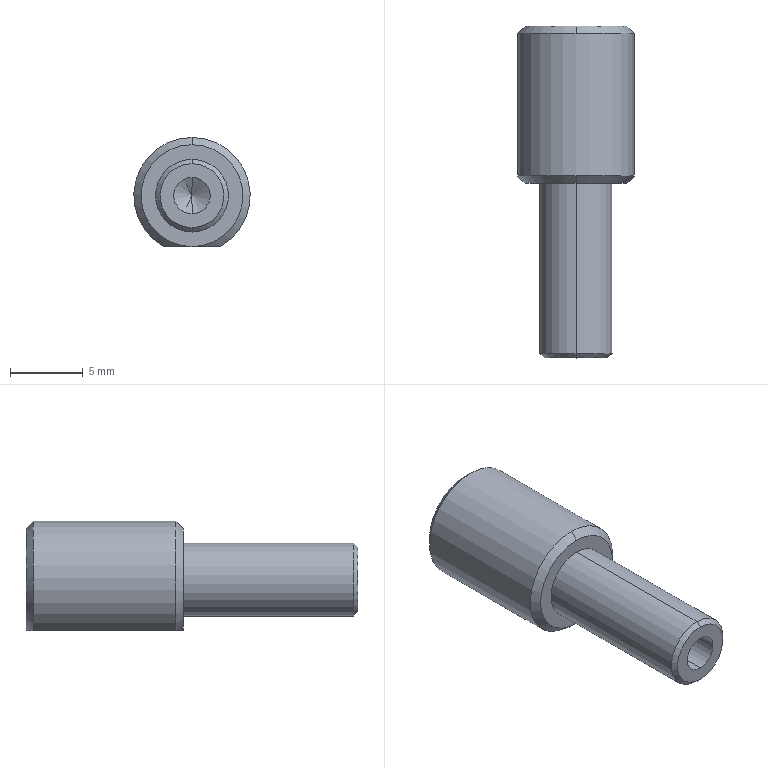Part | SolidWorks | features Chamfer 2, Cut 1, Extrusion 1, HoleWzd 1, ICE 1 | 1 solid | 17 faces | box 8 x 22.8 x 7.5 mm | volume 720.407 mm3 | cone 8 | cylinder 5 | plane 4 | commonest cylinder face diameters 2.5 x2 5 x2 8 x1
STEP:
#1=CARTESIAN_POINT('',(0.,7.5,1.25));
#2=VERTEX_POINT('',#1);
#3=CARTESIAN_POINT('',(0.,7.5,-1.25));
#4=VERTEX_POINT('',#3);
#5=CARTESIAN_POINT('',(0.,7.5,0.));
#6=DIRECTION('',(0.,-1.,0.));
#7=DIRECTION('',(0.,0.,-1.));
#8=AXIS2_PLACEMENT_3D('',#5,#6,#7);
#9=CIRCLE('',#8,1.25);
#10=EDGE_CURVE('',#2,#4,#9,.T.);
#11=ORIENTED_EDGE('',*,*,#10,.F.);
#12=CARTESIAN_POINT('',(0.,0.,1.25));
#13=VERTEX_POINT('',#12);
#14=CARTESIAN_POINT('',(0.,0.,1.25));
#15=DIRECTION('',(0.,-1.,0.));
#16=VECTOR('',#15,1000.);
#17=LINE('',#14,#16);
#18=EDGE_CURVE('',#2,#13,#17,.T.);
#19=ORIENTED_EDGE('',*,*,#18,.T.);
#20=CARTESIAN_POINT('',(0.,0.,-1.25));
#21=VERTEX_POINT('',#20);
#22=CARTESIAN_POINT('',(0.,0.,0.));
#23=DIRECTION('',(0.,-1.,0.));
#24=DIRECTION('',(0.,0.,-1.));
#25=AXIS2_PLACEMENT_3D('',#22,#23,#24);
#26=CIRCLE('',#25,1.25);
#27=EDGE_CURVE('',#13,#21,#26,.T.);
#28=ORIENTED_EDGE('',*,*,#27,.T.);
#29=CARTESIAN_POINT('',(0.,0.,-1.25));
#30=DIRECTION('',(0.,-1.,0.));
#31=VECTOR('',#30,1000.);
#32=LINE('',#29,#31);
#33=EDGE_CURVE('',#4,#21,#32,.T.);
#34=ORIENTED_EDGE('',*,*,#33,.F.);
#35=EDGE_LOOP('',(#11,#19,#28,#34));
#36=FACE_OUTER_BOUND('',#35,.T.);
#37=CARTESIAN_POINT('',(0.,0.,0.));
#38=DIRECTION('',(0.,-1.,0.));
#39=DIRECTION('',(0.,0.,-1.));
#40=AXIS2_PLACEMENT_3D('',#37,#38,#39);
#41=CYLINDRICAL_SURFACE('',#40,1.25);
#42=ADVANCED_FACE('',(#36),#41,.F.);
#43=CARTESIAN_POINT('',(0.,8.251,0.));
#44=VERTEX_POINT('',#43);
#45=CARTESIAN_POINT('',(0.,7.5,-1.25));
#46=DIRECTION('',(0.,-0.515,-0.8572));
#47=VECTOR('',#46,1000.);
#48=LINE('',#45,#47);
#49=EDGE_CURVE('',#44,#4,#48,.T.);
#50=ORIENTED_EDGE('',*,*,#49,.F.);
#51=CARTESIAN_POINT('',(0.,7.5,1.25));
#52=DIRECTION('',(0.,-0.515,0.8572));
#53=VECTOR('',#52,1000.);
#54=LINE('',#51,#53);
#55=EDGE_CURVE('',#44,#2,#54,.T.);
#56=ORIENTED_EDGE('',*,*,#55,.T.);
#57=ORIENTED_EDGE('',*,*,#10,.T.);
#58=EDGE_LOOP('',(#50,#56,#57));
#59=FACE_OUTER_BOUND('',#58,.T.);
#60=CARTESIAN_POINT('',(0.,7.5,0.));
#61=DIRECTION('',(0.,-1.,0.));
#62=DIRECTION('',(0.,0.,-1.));
#63=AXIS2_PLACEMENT_3D('',#60,#61,#62);
#64=CONICAL_SURFACE('',#63,1.25,1.03);
#65=ADVANCED_FACE('',(#59),#64,.F.);
#66=CARTESIAN_POINT('',(0.,0.,-2.2));
#67=VERTEX_POINT('',#66);
#68=CARTESIAN_POINT('',(0.,0.,2.2));
#69=VERTEX_POINT('',#68);
#70=CARTESIAN_POINT('',(0.,0.,0.));
#71=DIRECTION('',(0.,-1.,0.));
#72=DIRECTION('',(0.,0.,1.));
#73=AXIS2_PLACEMENT_3D('',#70,#71,#72);
#74=CIRCLE('',#73,2.2);
#75=EDGE_CURVE('',#67,#69,#74,.T.);
#76=ORIENTED_EDGE('',*,*,#75,.F.);
#77=CARTESIAN_POINT('',(0.,0.3,-2.5));
#78=VERTEX_POINT('',#77);
#79=CARTESIAN_POINT('',(0.,0.3,-2.5));
#80=DIRECTION('',(0.,0.7071,-0.7071));
#81=VECTOR('',#80,1000.);
#82=LINE('',#79,#81);
#83=EDGE_CURVE('',#67,#78,#82,.T.);
#84=ORIENTED_EDGE('',*,*,#83,.T.);
#85=CARTESIAN_POINT('',(0.,0.3,2.5));
#86=VERTEX_POINT('',#85);
#87=CARTESIAN_POINT('',(0.,0.3,0.));
#88=DIRECTION('',(0.,1.,0.));
#89=DIRECTION('',(0.,0.,1.));
#90=AXIS2_PLACEMENT_3D('',#87,#88,#89);
#91=CIRCLE('',#90,2.5);
#92=EDGE_CURVE('',#86,#78,#91,.T.);
#93=ORIENTED_EDGE('',*,*,#92,.F.);
#94=CARTESIAN_POINT('',(0.,0.3,2.5));
#95=DIRECTION('',(0.,0.7071,0.7071));
#96=VECTOR('',#95,1000.);
#97=LINE('',#94,#96);
#98=EDGE_CURVE('',#69,#86,#97,.T.);
#99=ORIENTED_EDGE('',*,*,#98,.F.);
#100=EDGE_LOOP('',(#76,#84,#93,#99));
#101=FACE_OUTER_BOUND('',#100,.T.);
#102=CARTESIAN_POINT('',(0.,0.3,0.));
#103=DIRECTION('',(0.,1.,0.));
#104=DIRECTION('',(0.,0.,1.));
#105=AXIS2_PLACEMENT_3D('',#102,#103,#104);
#106=CONICAL_SURFACE('',#105,2.5,0.7854);
#107=ADVANCED_FACE('',(#101),#106,.T.);
#108=CARTESIAN_POINT('',(0.,12.,3.5));
#109=VERTEX_POINT('',#108);
#110=CARTESIAN_POINT('',(0.,12.,-3.5));
#111=VERTEX_POINT('',#110);
#112=CARTESIAN_POINT('',(0.,12.,0.));
#113=DIRECTION('',(0.,-1.,0.));
#114=DIRECTION('',(0.,0.,1.));
#115=AXIS2_PLACEMENT_3D('',#112,#113,#114);
#116=CIRCLE('',#115,3.5);
#117=EDGE_CURVE('',#109,#111,#116,.T.);
#118=ORIENTED_EDGE('',*,*,#117,.F.);
#119=CARTESIAN_POINT('',(0.,12.5,4.));
#120=VERTEX_POINT('',#119);
#121=CARTESIAN_POINT('',(0.,12.5,4.));
#122=DIRECTION('',(0.,0.7071,0.7071));
#123=VECTOR('',#122,1000.);
#124=LINE('',#121,#123);
#125=EDGE_CURVE('',#109,#120,#124,.T.);
#126=ORIENTED_EDGE('',*,*,#125,.T.);
#127=CARTESIAN_POINT('',(-1.936,12.5,-3.5));
#128=VERTEX_POINT('',#127);
#129=CARTESIAN_POINT('',(0.,12.5,0.));
#130=DIRECTION('',(0.,1.,0.));
#131=DIRECTION('',(0.,0.,1.));
#132=AXIS2_PLACEMENT_3D('',#129,#130,#131);
#133=CIRCLE('',#132,4.);
#134=EDGE_CURVE('',#128,#120,#133,.T.);
#135=ORIENTED_EDGE('',*,*,#134,.F.);
#136=CARTESIAN_POINT('',(0.,12.,-3.5));
#137=CARTESIAN_POINT('',(-0.34,12.,-3.5));
#138=CARTESIAN_POINT('',(-0.673,12.05,-3.5));
#139=CARTESIAN_POINT('',(-1.328,12.23,-3.5));
#140=CARTESIAN_POINT('',(-1.638,12.355,-3.5));
#141=CARTESIAN_POINT('',(-1.936,12.5,-3.5));
#142=B_SPLINE_CURVE_WITH_KNOTS('',3,(#136,#137,#138,#139,#140,#141),.UNSPECIFIED.,.F.,.F.,(4,2,4),(0.004182,0.005183,0.006184),.UNSPECIFIED.);
#143=EDGE_CURVE('',#111,#128,#142,.T.);
#144=ORIENTED_EDGE('',*,*,#143,.F.);
#145=EDGE_LOOP('',(#118,#126,#135,#144));
#146=FACE_OUTER_BOUND('',#145,.T.);
#147=CARTESIAN_POINT('',(0.,12.5,0.));
#148=DIRECTION('',(0.,1.,0.));
#149=DIRECTION('',(0.,0.,1.));
#150=AXIS2_PLACEMENT_3D('',#147,#148,#149);
#151=CONICAL_SURFACE('',#150,4.,0.7854);
#152=ADVANCED_FACE('',(#146),#151,.T.);
#153=CARTESIAN_POINT('',(0.,22.8,3.5));
#154=VERTEX_POINT('',#153);
#155=CARTESIAN_POINT('',(0.,22.8,-3.5));
#156=VERTEX_POINT('',#155);
#157=CARTESIAN_POINT('',(0.,22.8,0.));
#158=DIRECTION('',(0.,1.,0.));
#159=DIRECTION('',(0.,0.,1.));
#160=AXIS2_PLACEMENT_3D('',#157,#158,#159);
#161=CIRCLE('',#160,3.5);
#162=EDGE_CURVE('',#154,#156,#161,.T.);
#163=ORIENTED_EDGE('',*,*,#162,.F.);
#164=CARTESIAN_POINT('',(0.,22.3,4.));
#165=VERTEX_POINT('',#164);
#166=CARTESIAN_POINT('',(0.,22.8,3.5));
#167=DIRECTION('',(0.,-0.7071,0.7071));
#168=VECTOR('',#167,1000.);
#169=LINE('',#166,#168);
#170=EDGE_CURVE('',#154,#165,#169,.T.);
#171=ORIENTED_EDGE('',*,*,#170,.T.);
#172=CARTESIAN_POINT('',(1.936,22.3,-3.5));
#173=VERTEX_POINT('',#172);
#174=CARTESIAN_POINT('',(0.,22.3,0.));
#175=DIRECTION('',(0.,-1.,0.));
#176=DIRECTION('',(0.,0.,1.));
#177=AXIS2_PLACEMENT_3D('',#174,#175,#176);
#178=CIRCLE('',#177,4.);
#179=EDGE_CURVE('',#173,#165,#178,.T.);
#180=ORIENTED_EDGE('',*,*,#179,.F.);
#181=CARTESIAN_POINT('',(0.,22.8,-3.5));
#182=CARTESIAN_POINT('',(0.3393,22.8,-3.5));
#183=CARTESIAN_POINT('',(0.6719,22.75,-3.5));
#184=CARTESIAN_POINT('',(1.158,22.617,-3.5));
#185=CARTESIAN_POINT('',(1.319,22.562,-3.5));
#186=CARTESIAN_POINT('',(1.633,22.44,-3.5));
#187=CARTESIAN_POINT('',(1.786,22.373,-3.5));
#188=CARTESIAN_POINT('',(1.936,22.3,-3.5));
#189=B_SPLINE_CURVE_WITH_KNOTS('',3,(#181,#182,#183,#184,#185,#186,#187,#188),.UNSPECIFIED.,.F.,.F.,(4,2,2,4),(0.01206,0.01306,0.01356,0.01406),.UNSPECIFIED.);
#190=EDGE_CURVE('',#156,#173,#189,.T.);
#191=ORIENTED_EDGE('',*,*,#190,.F.);
#192=EDGE_LOOP('',(#163,#171,#180,#191));
#193=FACE_OUTER_BOUND('',#192,.T.);
#194=CARTESIAN_POINT('',(0.,22.8,0.));
#195=DIRECTION('',(0.,-1.,0.));
#196=DIRECTION('',(0.,0.,-1.));
#197=AXIS2_PLACEMENT_3D('',#194,#195,#196);
#198=CONICAL_SURFACE('',#197,3.5,0.7854);
#199=ADVANCED_FACE('',(#193),#198,.T.);
#200=CARTESIAN_POINT('',(0.,12.,2.5));
#201=VERTEX_POINT('',#200);
#202=CARTESIAN_POINT('',(0.,12.,-2.5));
#203=VERTEX_POINT('',#202);
#204=CARTESIAN_POINT('',(0.,12.,0.));
#205=DIRECTION('',(0.,1.,0.));
#206=DIRECTION('',(0.,0.,1.));
#207=AXIS2_PLACEMENT_3D('',#204,#205,#206);
#208=CIRCLE('',#207,2.5);
#209=EDGE_CURVE('',#201,#203,#208,.T.);
#210=ORIENTED_EDGE('',*,*,#209,.F.);
#211=CARTESIAN_POINT('',(0.,12.,2.5));
#212=DIRECTION('',(0.,-1.,0.));
#213=VECTOR('',#212,1000.);
#214=LINE('',#211,#213);
#215=EDGE_CURVE('',#201,#86,#214,.T.);
#216=ORIENTED_EDGE('',*,*,#215,.T.);
#217=ORIENTED_EDGE('',*,*,#92,.T.);
#218=CARTESIAN_POINT('',(0.,12.,-2.5));
#219=DIRECTION('',(0.,-1.,0.));
#220=VECTOR('',#219,1000.);
#221=LINE('',#218,#220);
#222=EDGE_CURVE('',#203,#78,#221,.T.);
#223=ORIENTED_EDGE('',*,*,#222,.F.);
#224=EDGE_LOOP('',(#210,#216,#217,#223));
#225=FACE_OUTER_BOUND('',#224,.T.);
#226=CARTESIAN_POINT('',(0.,12.,0.));
#227=DIRECTION('',(0.,-1.,0.));
#228=DIRECTION('',(0.,0.,-1.));
#229=AXIS2_PLACEMENT_3D('',#226,#227,#228);
#230=CYLINDRICAL_SURFACE('',#229,2.5);
#231=ADVANCED_FACE('',(#225),#230,.T.);
#232=ORIENTED_EDGE('',*,*,#215,.F.);
#233=CARTESIAN_POINT('',(0.,12.,0.));
#234=DIRECTION('',(0.,1.,0.));
#235=DIRECTION('',(0.,0.,1.));
#236=AXIS2_PLACEMENT_3D('',#233,#234,#235);
#237=CIRCLE('',#236,2.5);
#238=EDGE_CURVE('',#203,#201,#237,.T.);
#239=ORIENTED_EDGE('',*,*,#238,.F.);
#240=ORIENTED_EDGE('',*,*,#222,.T.);
#241=CARTESIAN_POINT('',(0.,0.3,0.));
#242=DIRECTION('',(0.,1.,0.));
#243=DIRECTION('',(0.,0.,1.));
#244=AXIS2_PLACEMENT_3D('',#241,#242,#243);
#245=CIRCLE('',#244,2.5);
#246=EDGE_CURVE('',#78,#86,#245,.T.);
#247=ORIENTED_EDGE('',*,*,#246,.T.);
#248=EDGE_LOOP('',(#232,#239,#240,#247));
#249=FACE_OUTER_BOUND('',#248,.T.);
#250=CARTESIAN_POINT('',(0.,12.,0.));
#251=DIRECTION('',(0.,-1.,0.));
#252=DIRECTION('',(0.,0.,-1.));
#253=AXIS2_PLACEMENT_3D('',#250,#251,#252);
#254=CYLINDRICAL_SURFACE('',#253,2.5);
#255=ADVANCED_FACE('',(#249),#254,.T.);
#256=CARTESIAN_POINT('',(0.,0.,0.));
#257=DIRECTION('',(0.,-1.,0.));
#258=DIRECTION('',(0.,0.,-1.));
#259=AXIS2_PLACEMENT_3D('',#256,#257,#258);
#260=CIRCLE('',#259,1.25);
#261=EDGE_CURVE('',#21,#13,#260,.T.);
#262=ORIENTED_EDGE('',*,*,#261,.F.);
#263=ORIENTED_EDGE('',*,*,#27,.F.);
#264=EDGE_LOOP('',(#262,#263));
#265=FACE_BOUND('',#264,.T.);
#266=CARTESIAN_POINT('',(0.,0.,0.));
#267=DIRECTION('',(0.,-1.,0.));
#268=DIRECTION('',(0.,0.,1.));
#269=AXIS2_PLACEMENT_3D('',#266,#267,#268);
#270=CIRCLE('',#269,2.2);
#271=EDGE_CURVE('',#69,#67,#270,.T.);
#272=ORIENTED_EDGE('',*,*,#271,.T.);
#273=ORIENTED_EDGE('',*,*,#75,.T.);
#274=EDGE_LOOP('',(#272,#273));
#275=FACE_OUTER_BOUND('',#274,.T.);
#276=CARTESIAN_POINT('',(0.,0.,0.));
#277=DIRECTION('',(0.,1.,0.));
#278=DIRECTION('',(0.,0.,1.));
#279=AXIS2_PLACEMENT_3D('',#276,#277,#278);
#280=PLANE('',#279);
#281=ADVANCED_FACE('',(#265,#275),#280,.F.);
#282=CARTESIAN_POINT('',(0.,12.,0.));
#283=DIRECTION('',(0.,-1.,0.));
#284=DIRECTION('',(0.,0.,1.));
#285=AXIS2_PLACEMENT_3D('',#282,#283,#284);
#286=CIRCLE('',#285,3.5);
#287=EDGE_CURVE('',#111,#109,#286,.T.);
#288=ORIENTED_EDGE('',*,*,#287,.T.);
#289=ORIENTED_EDGE('',*,*,#117,.T.);
#290=EDGE_LOOP('',(#288,#289));
#291=FACE_OUTER_BOUND('',#290,.T.);
#292=ORIENTED_EDGE('',*,*,#238,.T.);
#293=ORIENTED_EDGE('',*,*,#209,.T.);
#294=EDGE_LOOP('',(#292,#293));
#295=FACE_BOUND('',#294,.T.);
#296=CARTESIAN_POINT('',(0.,12.,0.));
#297=DIRECTION('',(0.,1.,0.));
#298=DIRECTION('',(0.,0.,1.));
#299=AXIS2_PLACEMENT_3D('',#296,#297,#298);
#300=PLANE('',#299);
#301=ADVANCED_FACE('',(#291,#295),#300,.F.);
#302=ORIENTED_EDGE('',*,*,#179,.T.);
#303=CARTESIAN_POINT('',(-1.936,22.3,-3.5));
#304=VERTEX_POINT('',#303);
#305=CARTESIAN_POINT('',(0.,22.3,0.));
#306=DIRECTION('',(0.,-1.,0.));
#307=DIRECTION('',(0.,0.,1.));
#308=AXIS2_PLACEMENT_3D('',#305,#306,#307);
#309=CIRCLE('',#308,4.);
#310=EDGE_CURVE('',#165,#304,#309,.T.);
#311=ORIENTED_EDGE('',*,*,#310,.T.);
#312=CARTESIAN_POINT('',(-1.936,22.8,-3.5));
#313=DIRECTION('',(0.,-1.,0.));
#314=VECTOR('',#313,1000.);
#315=LINE('',#312,#314);
#316=EDGE_CURVE('',#304,#128,#315,.T.);
#317=ORIENTED_EDGE('',*,*,#316,.T.);
#318=ORIENTED_EDGE('',*,*,#134,.T.);
#319=CARTESIAN_POINT('',(1.936,12.5,-3.5));
#320=VERTEX_POINT('',#319);
#321=CARTESIAN_POINT('',(0.,12.5,0.));
#322=DIRECTION('',(0.,1.,0.));
#323=DIRECTION('',(0.,0.,1.));
#324=AXIS2_PLACEMENT_3D('',#321,#322,#323);
#325=CIRCLE('',#324,4.);
#326=EDGE_CURVE('',#120,#320,#325,.T.);
#327=ORIENTED_EDGE('',*,*,#326,.T.);
#328=CARTESIAN_POINT('',(1.936,22.8,-3.5));
#329=DIRECTION('',(0.,1.,0.));
#330=VECTOR('',#329,1000.);
#331=LINE('',#328,#330);
#332=EDGE_CURVE('',#320,#173,#331,.T.);
#333=ORIENTED_EDGE('',*,*,#332,.T.);
#334=EDGE_LOOP('',(#302,#311,#317,#318,#327,#333));
#335=FACE_OUTER_BOUND('',#334,.T.);
#336=CARTESIAN_POINT('',(0.,22.8,0.));
#337=DIRECTION('',(0.,-1.,0.));
#338=DIRECTION('',(0.,0.,-1.));
#339=AXIS2_PLACEMENT_3D('',#336,#337,#338);
#340=CYLINDRICAL_SURFACE('',#339,4.);
#341=ADVANCED_FACE('',(#335),#340,.T.);
#342=CARTESIAN_POINT('',(0.,22.8,0.));
#343=DIRECTION('',(0.,1.,0.));
#344=DIRECTION('',(0.,0.,1.));
#345=AXIS2_PLACEMENT_3D('',#342,#343,#344);
#346=CIRCLE('',#345,3.5);
#347=EDGE_CURVE('',#156,#154,#346,.T.);
#348=ORIENTED_EDGE('',*,*,#347,.T.);
#349=ORIENTED_EDGE('',*,*,#162,.T.);
#350=EDGE_LOOP('',(#348,#349));
#351=FACE_OUTER_BOUND('',#350,.T.);
#352=CARTESIAN_POINT('',(0.,22.8,0.));
#353=DIRECTION('',(0.,1.,0.));
#354=DIRECTION('',(0.,0.,1.));
#355=AXIS2_PLACEMENT_3D('',#352,#353,#354);
#356=PLANE('',#355);
#357=ADVANCED_FACE('',(#351),#356,.T.);
#358=ORIENTED_EDGE('',*,*,#170,.F.);
#359=ORIENTED_EDGE('',*,*,#347,.F.);
#360=CARTESIAN_POINT('',(-1.936,22.3,-3.5));
#361=CARTESIAN_POINT('',(-1.638,22.445,-3.5));
#362=CARTESIAN_POINT('',(-1.328,22.57,-3.5));
#363=CARTESIAN_POINT('',(-0.673,22.75,-3.5));
#364=CARTESIAN_POINT('',(-0.34,22.8,-3.5));
#365=CARTESIAN_POINT('',(0.,22.8,-3.5));
#366=B_SPLINE_CURVE_WITH_KNOTS('',3,(#360,#361,#362,#363,#364,#365),.UNSPECIFIED.,.F.,.F.,(4,2,4),(0.01007,0.01107,0.01206),.UNSPECIFIED.);
#367=EDGE_CURVE('',#304,#156,#366,.T.);
#368=ORIENTED_EDGE('',*,*,#367,.F.);
#369=ORIENTED_EDGE('',*,*,#310,.F.);
#370=EDGE_LOOP('',(#358,#359,#368,#369));
#371=FACE_OUTER_BOUND('',#370,.T.);
#372=CARTESIAN_POINT('',(0.,22.8,0.));
#373=DIRECTION('',(0.,-1.,0.));
#374=DIRECTION('',(0.,0.,-1.));
#375=AXIS2_PLACEMENT_3D('',#372,#373,#374);
#376=CONICAL_SURFACE('',#375,3.5,0.7854);
#377=ADVANCED_FACE('',(#371),#376,.T.);
#378=ORIENTED_EDGE('',*,*,#125,.F.);
#379=ORIENTED_EDGE('',*,*,#287,.F.);
#380=CARTESIAN_POINT('',(1.936,12.5,-3.5));
#381=CARTESIAN_POINT('',(1.786,12.427,-3.5));
#382=CARTESIAN_POINT('',(1.633,12.36,-3.5));
#383=CARTESIAN_POINT('',(1.319,12.238,-3.5));
#384=CARTESIAN_POINT('',(1.158,12.183,-3.5));
#385=CARTESIAN_POINT('',(0.6719,12.05,-3.5));
#386=CARTESIAN_POINT('',(0.3393,12.,-3.5));
#387=CARTESIAN_POINT('',(0.,12.,-3.5));
#388=B_SPLINE_CURVE_WITH_KNOTS('',3,(#380,#381,#382,#383,#384,#385,#386,#387),.UNSPECIFIED.,.F.,.F.,(4,2,2,4),(0.002184,0.002684,0.003183,0.004182),.UNSPECIFIED.);
#389=EDGE_CURVE('',#320,#111,#388,.T.);
#390=ORIENTED_EDGE('',*,*,#389,.F.);
#391=ORIENTED_EDGE('',*,*,#326,.F.);
#392=EDGE_LOOP('',(#378,#379,#390,#391));
#393=FACE_OUTER_BOUND('',#392,.T.);
#394=CARTESIAN_POINT('',(0.,12.5,0.));
#395=DIRECTION('',(0.,1.,0.));
#396=DIRECTION('',(0.,0.,1.));
#397=AXIS2_PLACEMENT_3D('',#394,#395,#396);
#398=CONICAL_SURFACE('',#397,4.,0.7854);
#399=ADVANCED_FACE('',(#393),#398,.T.);
#400=ORIENTED_EDGE('',*,*,#83,.F.);
#401=ORIENTED_EDGE('',*,*,#271,.F.);
#402=ORIENTED_EDGE('',*,*,#98,.T.);
#403=ORIENTED_EDGE('',*,*,#246,.F.);
#404=EDGE_LOOP('',(#400,#401,#402,#403));
#405=FACE_OUTER_BOUND('',#404,.T.);
#406=CARTESIAN_POINT('',(0.,0.3,0.));
#407=DIRECTION('',(0.,1.,0.));
#408=DIRECTION('',(0.,0.,1.));
#409=AXIS2_PLACEMENT_3D('',#406,#407,#408);
#410=CONICAL_SURFACE('',#409,2.5,0.7854);
#411=ADVANCED_FACE('',(#405),#410,.T.);
#412=ORIENTED_EDGE('',*,*,#367,.T.);
#413=ORIENTED_EDGE('',*,*,#190,.T.);
#414=ORIENTED_EDGE('',*,*,#332,.F.);
#415=ORIENTED_EDGE('',*,*,#389,.T.);
#416=ORIENTED_EDGE('',*,*,#143,.T.);
#417=ORIENTED_EDGE('',*,*,#316,.F.);
#418=EDGE_LOOP('',(#412,#413,#414,#415,#416,#417));
#419=FACE_OUTER_BOUND('',#418,.T.);
#420=CARTESIAN_POINT('',(-4.,10.8,-3.5));
#421=DIRECTION('',(0.,0.,1.));
#422=DIRECTION('',(1.,0.,0.));
#423=AXIS2_PLACEMENT_3D('',#420,#421,#422);
#424=PLANE('',#423);
#425=ADVANCED_FACE('',(#419),#424,.F.);
#426=ORIENTED_EDGE('',*,*,#55,.F.);
#427=ORIENTED_EDGE('',*,*,#49,.T.);
#428=CARTESIAN_POINT('',(0.,7.5,0.));
#429=DIRECTION('',(0.,-1.,0.));
#430=DIRECTION('',(0.,0.,-1.));
#431=AXIS2_PLACEMENT_3D('',#428,#429,#430);
#432=CIRCLE('',#431,1.25);
#433=EDGE_CURVE('',#4,#2,#432,.T.);
#434=ORIENTED_EDGE('',*,*,#433,.T.);
#435=EDGE_LOOP('',(#426,#427,#434));
#436=FACE_OUTER_BOUND('',#435,.T.);
#437=CARTESIAN_POINT('',(0.,7.5,0.));
#438=DIRECTION('',(0.,-1.,0.));
#439=DIRECTION('',(0.,0.,-1.));
#440=AXIS2_PLACEMENT_3D('',#437,#438,#439);
#441=CONICAL_SURFACE('',#440,1.25,1.03);
#442=ADVANCED_FACE('',(#436),#441,.F.);
#443=ORIENTED_EDGE('',*,*,#18,.F.);
#444=ORIENTED_EDGE('',*,*,#433,.F.);
#445=ORIENTED_EDGE('',*,*,#33,.T.);
#446=ORIENTED_EDGE('',*,*,#261,.T.);
#447=EDGE_LOOP('',(#443,#444,#445,#446));
#448=FACE_OUTER_BOUND('',#447,.T.);
#449=CARTESIAN_POINT('',(0.,0.,0.));
#450=DIRECTION('',(0.,-1.,0.));
#451=DIRECTION('',(0.,0.,-1.));
#452=AXIS2_PLACEMENT_3D('',#449,#450,#451);
#453=CYLINDRICAL_SURFACE('',#452,1.25);
#454=ADVANCED_FACE('',(#448),#453,.F.);
#455=CLOSED_SHELL('',(#42,#65,#107,#152,#199,#231,#255,#281,#301,#341,#357,#377,#399,#411,#425,#442,#454));
#456=MANIFOLD_SOLID_BREP('',#455);
#457=CARTESIAN_POINT('',(0.,0.,0.));
#458=DIRECTION('',(0.,0.,1.));
#459=DIRECTION('',(1.,0.,0.));
#460=AXIS2_PLACEMENT_3D('',#457,#458,#459);
#461=(LENGTH_UNIT()NAMED_UNIT(*)SI_UNIT(.MILLI.,.METRE.));
#462=UNCERTAINTY_MEASURE_WITH_UNIT(LENGTH_MEASURE(0.00001),#461,'','');
#463=(NAMED_UNIT(*)PLANE_ANGLE_UNIT()SI_UNIT($,.RADIAN.));
#464=(NAMED_UNIT(*)SI_UNIT($,.STERADIAN.)SOLID_ANGLE_UNIT());
#465=(GEOMETRIC_REPRESENTATION_CONTEXT(3)GLOBAL_UNCERTAINTY_ASSIGNED_CONTEXT((#462))GLOBAL_UNIT_ASSIGNED_CONTEXT((#461,#463,#464))REPRESENTATION_CONTEXT('',''));
#466=ADVANCED_BREP_SHAPE_REPRESENTATION('',(#456,#460),#465);